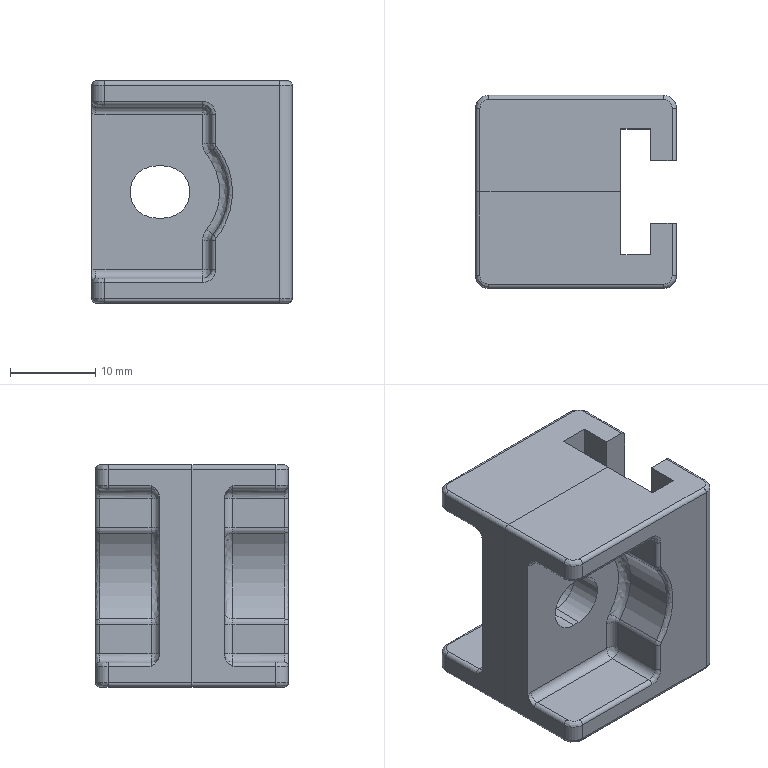Part | SolidWorks | features BaseBody 2 | 2 solids | 142 faces | box 23.5 x 22.6 x 26 mm | volume 7127 mm3 | cylinder 60 | spline 38 | plane 38 | cone 4 | torus 2 | commonest cylinder face diameters 1 x24 2 x16 3 x6 5 x4 5.1 x4 6.1 x4